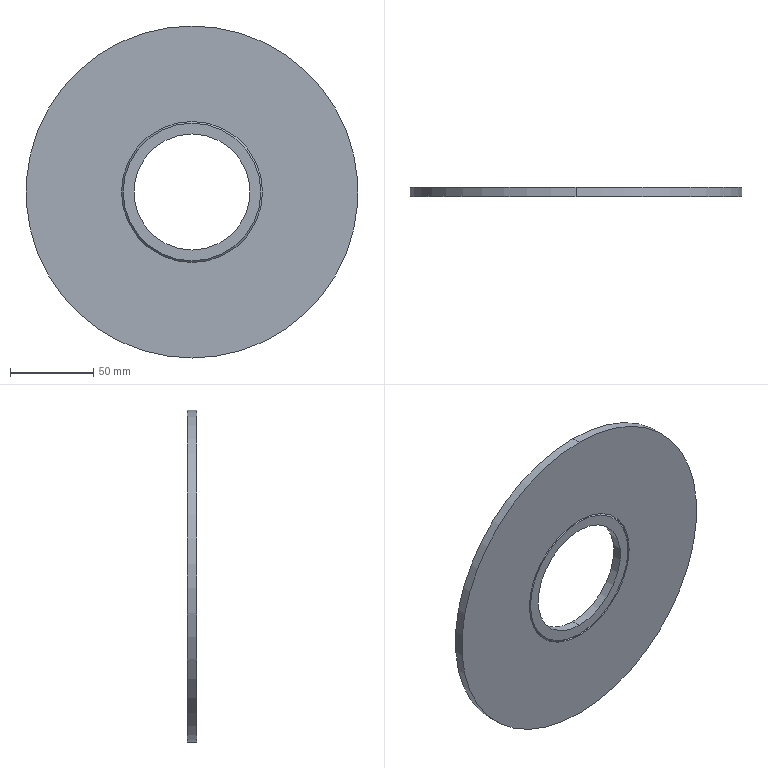Part | SolidWorks | features Chamfer 1, Extrusion 1, ICE 1 | 1 solid | 16 faces | box 200 x 5.5 x 200 mm | volume 151356 mm3 | cylinder 8 | cone 4 | plane 4 | commonest cylinder face diameters 85 x4 70 x2 200 x2
STEP:
#1=CARTESIAN_POINT('',(0.,4.5,42.5));
#2=VERTEX_POINT('',#1);
#3=CARTESIAN_POINT('',(0.,4.5,-42.5));
#4=VERTEX_POINT('',#3);
#5=CARTESIAN_POINT('',(0.,4.5,0.));
#6=DIRECTION('',(0.,-1.,0.));
#7=DIRECTION('',(0.,0.,1.));
#8=AXIS2_PLACEMENT_3D('',#5,#6,#7);
#9=CIRCLE('',#8,42.5);
#10=EDGE_CURVE('',#2,#4,#9,.T.);
#11=ORIENTED_EDGE('',*,*,#10,.T.);
#12=CARTESIAN_POINT('',(0.,5.5,-42.5));
#13=VERTEX_POINT('',#12);
#14=CARTESIAN_POINT('',(0.,0.,-42.5));
#15=DIRECTION('',(0.,1.,0.));
#16=VECTOR('',#15,1000.);
#17=LINE('',#14,#16);
#18=EDGE_CURVE('',#4,#13,#17,.T.);
#19=ORIENTED_EDGE('',*,*,#18,.T.);
#20=CARTESIAN_POINT('',(0.,5.5,42.5));
#21=VERTEX_POINT('',#20);
#22=CARTESIAN_POINT('',(0.,5.5,0.));
#23=DIRECTION('',(0.,1.,0.));
#24=DIRECTION('',(0.,0.,1.));
#25=AXIS2_PLACEMENT_3D('',#22,#23,#24);
#26=CIRCLE('',#25,42.5);
#27=EDGE_CURVE('',#13,#21,#26,.T.);
#28=ORIENTED_EDGE('',*,*,#27,.T.);
#29=CARTESIAN_POINT('',(0.,0.,42.5));
#30=DIRECTION('',(0.,1.,0.));
#31=VECTOR('',#30,1000.);
#32=LINE('',#29,#31);
#33=EDGE_CURVE('',#2,#21,#32,.T.);
#34=ORIENTED_EDGE('',*,*,#33,.F.);
#35=EDGE_LOOP('',(#11,#19,#28,#34));
#36=FACE_OUTER_BOUND('',#35,.T.);
#37=CARTESIAN_POINT('',(0.,0.,0.));
#38=DIRECTION('',(0.,1.,0.));
#39=DIRECTION('',(0.,0.,1.));
#40=AXIS2_PLACEMENT_3D('',#37,#38,#39);
#41=CYLINDRICAL_SURFACE('',#40,42.5);
#42=ADVANCED_FACE('',(#36),#41,.F.);
#43=CARTESIAN_POINT('',(0.,0.,100.));
#44=VERTEX_POINT('',#43);
#45=CARTESIAN_POINT('',(0.,0.,-100.));
#46=VERTEX_POINT('',#45);
#47=CARTESIAN_POINT('',(0.,0.,0.));
#48=DIRECTION('',(0.,1.,0.));
#49=DIRECTION('',(0.,0.,1.));
#50=AXIS2_PLACEMENT_3D('',#47,#48,#49);
#51=CIRCLE('',#50,100.);
#52=EDGE_CURVE('',#44,#46,#51,.T.);
#53=ORIENTED_EDGE('',*,*,#52,.T.);
#54=CARTESIAN_POINT('',(0.,5.5,-100.));
#55=VERTEX_POINT('',#54);
#56=CARTESIAN_POINT('',(0.,0.,-100.));
#57=DIRECTION('',(0.,1.,0.));
#58=VECTOR('',#57,1000.);
#59=LINE('',#56,#58);
#60=EDGE_CURVE('',#46,#55,#59,.T.);
#61=ORIENTED_EDGE('',*,*,#60,.T.);
#62=CARTESIAN_POINT('',(0.,5.5,100.));
#63=VERTEX_POINT('',#62);
#64=CARTESIAN_POINT('',(0.,5.5,0.));
#65=DIRECTION('',(0.,1.,0.));
#66=DIRECTION('',(0.,0.,1.));
#67=AXIS2_PLACEMENT_3D('',#64,#65,#66);
#68=CIRCLE('',#67,100.);
#69=EDGE_CURVE('',#63,#55,#68,.T.);
#70=ORIENTED_EDGE('',*,*,#69,.F.);
#71=CARTESIAN_POINT('',(0.,0.,100.));
#72=DIRECTION('',(0.,1.,0.));
#73=VECTOR('',#72,1000.);
#74=LINE('',#71,#73);
#75=EDGE_CURVE('',#44,#63,#74,.T.);
#76=ORIENTED_EDGE('',*,*,#75,.F.);
#77=EDGE_LOOP('',(#53,#61,#70,#76));
#78=FACE_OUTER_BOUND('',#77,.T.);
#79=CARTESIAN_POINT('',(0.,0.,0.));
#80=DIRECTION('',(0.,1.,0.));
#81=DIRECTION('',(0.,0.,1.));
#82=AXIS2_PLACEMENT_3D('',#79,#80,#81);
#83=CYLINDRICAL_SURFACE('',#82,100.);
#84=ADVANCED_FACE('',(#78),#83,.T.);
#85=CARTESIAN_POINT('',(0.,0.,-42.5));
#86=VERTEX_POINT('',#85);
#87=CARTESIAN_POINT('',(0.,0.,42.5));
#88=VERTEX_POINT('',#87);
#89=CARTESIAN_POINT('',(0.,0.,0.));
#90=DIRECTION('',(0.,1.,0.));
#91=DIRECTION('',(0.,0.,1.));
#92=AXIS2_PLACEMENT_3D('',#89,#90,#91);
#93=CIRCLE('',#92,42.5);
#94=EDGE_CURVE('',#86,#88,#93,.T.);
#95=ORIENTED_EDGE('',*,*,#94,.F.);
#96=CARTESIAN_POINT('',(0.,1.,-42.5));
#97=VERTEX_POINT('',#96);
#98=CARTESIAN_POINT('',(0.,0.,-42.5));
#99=DIRECTION('',(0.,1.,0.));
#100=VECTOR('',#99,1000.);
#101=LINE('',#98,#100);
#102=EDGE_CURVE('',#86,#97,#101,.T.);
#103=ORIENTED_EDGE('',*,*,#102,.T.);
#104=CARTESIAN_POINT('',(0.,1.,42.5));
#105=VERTEX_POINT('',#104);
#106=CARTESIAN_POINT('',(0.,1.,0.));
#107=DIRECTION('',(0.,1.,0.));
#108=DIRECTION('',(0.,0.,1.));
#109=AXIS2_PLACEMENT_3D('',#106,#107,#108);
#110=CIRCLE('',#109,42.5);
#111=EDGE_CURVE('',#97,#105,#110,.T.);
#112=ORIENTED_EDGE('',*,*,#111,.T.);
#113=CARTESIAN_POINT('',(0.,0.,42.5));
#114=DIRECTION('',(0.,1.,0.));
#115=VECTOR('',#114,1000.);
#116=LINE('',#113,#115);
#117=EDGE_CURVE('',#88,#105,#116,.T.);
#118=ORIENTED_EDGE('',*,*,#117,.F.);
#119=EDGE_LOOP('',(#95,#103,#112,#118));
#120=FACE_OUTER_BOUND('',#119,.T.);
#121=CARTESIAN_POINT('',(0.,0.,0.));
#122=DIRECTION('',(0.,1.,0.));
#123=DIRECTION('',(0.,0.,1.));
#124=AXIS2_PLACEMENT_3D('',#121,#122,#123);
#125=CYLINDRICAL_SURFACE('',#124,42.5);
#126=ADVANCED_FACE('',(#120),#125,.F.);
#127=CARTESIAN_POINT('',(0.,5.5,41.5));
#128=VERTEX_POINT('',#127);
#129=CARTESIAN_POINT('',(0.,5.5,-41.5));
#130=VERTEX_POINT('',#129);
#131=CARTESIAN_POINT('',(0.,5.5,0.));
#132=DIRECTION('',(0.,1.,0.));
#133=DIRECTION('',(0.,0.,1.));
#134=AXIS2_PLACEMENT_3D('',#131,#132,#133);
#135=CIRCLE('',#134,41.5);
#136=EDGE_CURVE('',#128,#130,#135,.T.);
#137=ORIENTED_EDGE('',*,*,#136,.F.);
#138=CARTESIAN_POINT('',(0.,5.5,41.5));
#139=DIRECTION('',(0.,-0.7071,0.7071));
#140=VECTOR('',#139,1000.);
#141=LINE('',#138,#140);
#142=EDGE_CURVE('',#128,#2,#141,.T.);
#143=ORIENTED_EDGE('',*,*,#142,.T.);
#144=CARTESIAN_POINT('',(0.,4.5,0.));
#145=DIRECTION('',(0.,-1.,0.));
#146=DIRECTION('',(0.,0.,1.));
#147=AXIS2_PLACEMENT_3D('',#144,#145,#146);
#148=CIRCLE('',#147,42.5);
#149=EDGE_CURVE('',#4,#2,#148,.T.);
#150=ORIENTED_EDGE('',*,*,#149,.F.);
#151=CARTESIAN_POINT('',(0.,5.5,-41.5));
#152=DIRECTION('',(0.,-0.7071,-0.7071));
#153=VECTOR('',#152,1000.);
#154=LINE('',#151,#153);
#155=EDGE_CURVE('',#130,#4,#154,.T.);
#156=ORIENTED_EDGE('',*,*,#155,.F.);
#157=EDGE_LOOP('',(#137,#143,#150,#156));
#158=FACE_OUTER_BOUND('',#157,.T.);
#159=CARTESIAN_POINT('',(0.,5.5,0.));
#160=DIRECTION('',(0.,-1.,0.));
#161=DIRECTION('',(0.,0.,-1.));
#162=AXIS2_PLACEMENT_3D('',#159,#160,#161);
#163=CONICAL_SURFACE('',#162,41.5,0.7854);
#164=ADVANCED_FACE('',(#158),#163,.T.);
#165=CARTESIAN_POINT('',(0.,0.,-41.5));
#166=VERTEX_POINT('',#165);
#167=CARTESIAN_POINT('',(0.,0.,41.5));
#168=VERTEX_POINT('',#167);
#169=CARTESIAN_POINT('',(0.,0.,0.));
#170=DIRECTION('',(0.,-1.,0.));
#171=DIRECTION('',(0.,0.,1.));
#172=AXIS2_PLACEMENT_3D('',#169,#170,#171);
#173=CIRCLE('',#172,41.5);
#174=EDGE_CURVE('',#166,#168,#173,.T.);
#175=ORIENTED_EDGE('',*,*,#174,.F.);
#176=CARTESIAN_POINT('',(0.,1.,-42.5));
#177=DIRECTION('',(0.,0.7071,-0.7071));
#178=VECTOR('',#177,1000.);
#179=LINE('',#176,#178);
#180=EDGE_CURVE('',#166,#97,#179,.T.);
#181=ORIENTED_EDGE('',*,*,#180,.T.);
#182=CARTESIAN_POINT('',(0.,1.,0.));
#183=DIRECTION('',(0.,1.,0.));
#184=DIRECTION('',(0.,0.,1.));
#185=AXIS2_PLACEMENT_3D('',#182,#183,#184);
#186=CIRCLE('',#185,42.5);
#187=EDGE_CURVE('',#105,#97,#186,.T.);
#188=ORIENTED_EDGE('',*,*,#187,.F.);
#189=CARTESIAN_POINT('',(0.,1.,42.5));
#190=DIRECTION('',(0.,0.7071,0.7071));
#191=VECTOR('',#190,1000.);
#192=LINE('',#189,#191);
#193=EDGE_CURVE('',#168,#105,#192,.T.);
#194=ORIENTED_EDGE('',*,*,#193,.F.);
#195=EDGE_LOOP('',(#175,#181,#188,#194));
#196=FACE_OUTER_BOUND('',#195,.T.);
#197=CARTESIAN_POINT('',(0.,1.,0.));
#198=DIRECTION('',(0.,1.,0.));
#199=DIRECTION('',(0.,0.,1.));
#200=AXIS2_PLACEMENT_3D('',#197,#198,#199);
#201=CONICAL_SURFACE('',#200,42.5,0.7854);
#202=ADVANCED_FACE('',(#196),#201,.T.);
#203=CARTESIAN_POINT('',(0.,5.5,-35.));
#204=VERTEX_POINT('',#203);
#205=CARTESIAN_POINT('',(0.,5.5,35.));
#206=VERTEX_POINT('',#205);
#207=CARTESIAN_POINT('',(0.,5.5,0.));
#208=DIRECTION('',(0.,1.,0.));
#209=DIRECTION('',(0.,0.,1.));
#210=AXIS2_PLACEMENT_3D('',#207,#208,#209);
#211=CIRCLE('',#210,35.);
#212=EDGE_CURVE('',#204,#206,#211,.T.);
#213=ORIENTED_EDGE('',*,*,#212,.T.);
#214=CARTESIAN_POINT('',(0.,0.,35.));
#215=VERTEX_POINT('',#214);
#216=CARTESIAN_POINT('',(0.,5.5,35.));
#217=DIRECTION('',(0.,-1.,0.));
#218=VECTOR('',#217,1000.);
#219=LINE('',#216,#218);
#220=EDGE_CURVE('',#206,#215,#219,.T.);
#221=ORIENTED_EDGE('',*,*,#220,.T.);
#222=CARTESIAN_POINT('',(0.,0.,-35.));
#223=VERTEX_POINT('',#222);
#224=CARTESIAN_POINT('',(0.,0.,0.));
#225=DIRECTION('',(0.,1.,0.));
#226=DIRECTION('',(0.,0.,1.));
#227=AXIS2_PLACEMENT_3D('',#224,#225,#226);
#228=CIRCLE('',#227,35.);
#229=EDGE_CURVE('',#223,#215,#228,.T.);
#230=ORIENTED_EDGE('',*,*,#229,.F.);
#231=CARTESIAN_POINT('',(0.,5.5,-35.));
#232=DIRECTION('',(0.,-1.,0.));
#233=VECTOR('',#232,1000.);
#234=LINE('',#231,#233);
#235=EDGE_CURVE('',#204,#223,#234,.T.);
#236=ORIENTED_EDGE('',*,*,#235,.F.);
#237=EDGE_LOOP('',(#213,#221,#230,#236));
#238=FACE_OUTER_BOUND('',#237,.T.);
#239=CARTESIAN_POINT('',(0.,5.5,0.));
#240=DIRECTION('',(0.,-1.,0.));
#241=DIRECTION('',(0.,0.,-1.));
#242=AXIS2_PLACEMENT_3D('',#239,#240,#241);
#243=CYLINDRICAL_SURFACE('',#242,35.);
#244=ADVANCED_FACE('',(#238),#243,.F.);
#245=CARTESIAN_POINT('',(0.,5.5,0.));
#246=DIRECTION('',(0.,1.,0.));
#247=DIRECTION('',(0.,0.,1.));
#248=AXIS2_PLACEMENT_3D('',#245,#246,#247);
#249=CIRCLE('',#248,41.5);
#250=EDGE_CURVE('',#130,#128,#249,.T.);
#251=ORIENTED_EDGE('',*,*,#250,.T.);
#252=ORIENTED_EDGE('',*,*,#136,.T.);
#253=EDGE_LOOP('',(#251,#252));
#254=FACE_OUTER_BOUND('',#253,.T.);
#255=ORIENTED_EDGE('',*,*,#212,.F.);
#256=CARTESIAN_POINT('',(0.,5.5,0.));
#257=DIRECTION('',(0.,1.,0.));
#258=DIRECTION('',(0.,0.,1.));
#259=AXIS2_PLACEMENT_3D('',#256,#257,#258);
#260=CIRCLE('',#259,35.);
#261=EDGE_CURVE('',#206,#204,#260,.T.);
#262=ORIENTED_EDGE('',*,*,#261,.F.);
#263=EDGE_LOOP('',(#255,#262));
#264=FACE_BOUND('',#263,.T.);
#265=CARTESIAN_POINT('',(0.,5.5,0.));
#266=DIRECTION('',(0.,1.,0.));
#267=DIRECTION('',(0.,0.,1.));
#268=AXIS2_PLACEMENT_3D('',#265,#266,#267);
#269=PLANE('',#268);
#270=ADVANCED_FACE('',(#254,#264),#269,.T.);
#271=CARTESIAN_POINT('',(0.,0.,0.));
#272=DIRECTION('',(0.,-1.,0.));
#273=DIRECTION('',(0.,0.,1.));
#274=AXIS2_PLACEMENT_3D('',#271,#272,#273);
#275=CIRCLE('',#274,41.5);
#276=EDGE_CURVE('',#168,#166,#275,.T.);
#277=ORIENTED_EDGE('',*,*,#276,.T.);
#278=ORIENTED_EDGE('',*,*,#174,.T.);
#279=EDGE_LOOP('',(#277,#278));
#280=FACE_OUTER_BOUND('',#279,.T.);
#281=ORIENTED_EDGE('',*,*,#229,.T.);
#282=CARTESIAN_POINT('',(0.,0.,0.));
#283=DIRECTION('',(0.,1.,0.));
#284=DIRECTION('',(0.,0.,1.));
#285=AXIS2_PLACEMENT_3D('',#282,#283,#284);
#286=CIRCLE('',#285,35.);
#287=EDGE_CURVE('',#215,#223,#286,.T.);
#288=ORIENTED_EDGE('',*,*,#287,.T.);
#289=EDGE_LOOP('',(#281,#288));
#290=FACE_BOUND('',#289,.T.);
#291=CARTESIAN_POINT('',(0.,0.,0.));
#292=DIRECTION('',(0.,1.,0.));
#293=DIRECTION('',(0.,0.,1.));
#294=AXIS2_PLACEMENT_3D('',#291,#292,#293);
#295=PLANE('',#294);
#296=ADVANCED_FACE('',(#280,#290),#295,.F.);
#297=ORIENTED_EDGE('',*,*,#220,.F.);
#298=ORIENTED_EDGE('',*,*,#261,.T.);
#299=ORIENTED_EDGE('',*,*,#235,.T.);
#300=ORIENTED_EDGE('',*,*,#287,.F.);
#301=EDGE_LOOP('',(#297,#298,#299,#300));
#302=FACE_OUTER_BOUND('',#301,.T.);
#303=CARTESIAN_POINT('',(0.,5.5,0.));
#304=DIRECTION('',(0.,-1.,0.));
#305=DIRECTION('',(0.,0.,-1.));
#306=AXIS2_PLACEMENT_3D('',#303,#304,#305);
#307=CYLINDRICAL_SURFACE('',#306,35.);
#308=ADVANCED_FACE('',(#302),#307,.F.);
#309=ORIENTED_EDGE('',*,*,#180,.F.);
#310=ORIENTED_EDGE('',*,*,#276,.F.);
#311=ORIENTED_EDGE('',*,*,#193,.T.);
#312=ORIENTED_EDGE('',*,*,#111,.F.);
#313=EDGE_LOOP('',(#309,#310,#311,#312));
#314=FACE_OUTER_BOUND('',#313,.T.);
#315=CARTESIAN_POINT('',(0.,1.,0.));
#316=DIRECTION('',(0.,1.,0.));
#317=DIRECTION('',(0.,0.,1.));
#318=AXIS2_PLACEMENT_3D('',#315,#316,#317);
#319=CONICAL_SURFACE('',#318,42.5,0.7854);
#320=ADVANCED_FACE('',(#314),#319,.T.);
#321=ORIENTED_EDGE('',*,*,#142,.F.);
#322=ORIENTED_EDGE('',*,*,#250,.F.);
#323=ORIENTED_EDGE('',*,*,#155,.T.);
#324=ORIENTED_EDGE('',*,*,#10,.F.);
#325=EDGE_LOOP('',(#321,#322,#323,#324));
#326=FACE_OUTER_BOUND('',#325,.T.);
#327=CARTESIAN_POINT('',(0.,5.5,0.));
#328=DIRECTION('',(0.,-1.,0.));
#329=DIRECTION('',(0.,0.,-1.));
#330=AXIS2_PLACEMENT_3D('',#327,#328,#329);
#331=CONICAL_SURFACE('',#330,41.5,0.7854);
#332=ADVANCED_FACE('',(#326),#331,.T.);
#333=ORIENTED_EDGE('',*,*,#102,.F.);
#334=CARTESIAN_POINT('',(0.,0.,0.));
#335=DIRECTION('',(0.,1.,0.));
#336=DIRECTION('',(0.,0.,1.));
#337=AXIS2_PLACEMENT_3D('',#334,#335,#336);
#338=CIRCLE('',#337,42.5);
#339=EDGE_CURVE('',#88,#86,#338,.T.);
#340=ORIENTED_EDGE('',*,*,#339,.F.);
#341=ORIENTED_EDGE('',*,*,#117,.T.);
#342=ORIENTED_EDGE('',*,*,#187,.T.);
#343=EDGE_LOOP('',(#333,#340,#341,#342));
#344=FACE_OUTER_BOUND('',#343,.T.);
#345=CARTESIAN_POINT('',(0.,0.,0.));
#346=DIRECTION('',(0.,1.,0.));
#347=DIRECTION('',(0.,0.,1.));
#348=AXIS2_PLACEMENT_3D('',#345,#346,#347);
#349=CYLINDRICAL_SURFACE('',#348,42.5);
#350=ADVANCED_FACE('',(#344),#349,.F.);
#351=ORIENTED_EDGE('',*,*,#60,.F.);
#352=CARTESIAN_POINT('',(0.,0.,0.));
#353=DIRECTION('',(0.,1.,0.));
#354=DIRECTION('',(0.,0.,1.));
#355=AXIS2_PLACEMENT_3D('',#352,#353,#354);
#356=CIRCLE('',#355,100.);
#357=EDGE_CURVE('',#46,#44,#356,.T.);
#358=ORIENTED_EDGE('',*,*,#357,.T.);
#359=ORIENTED_EDGE('',*,*,#75,.T.);
#360=CARTESIAN_POINT('',(0.,5.5,0.));
#361=DIRECTION('',(0.,1.,0.));
#362=DIRECTION('',(0.,0.,1.));
#363=AXIS2_PLACEMENT_3D('',#360,#361,#362);
#364=CIRCLE('',#363,100.);
#365=EDGE_CURVE('',#55,#63,#364,.T.);
#366=ORIENTED_EDGE('',*,*,#365,.F.);
#367=EDGE_LOOP('',(#351,#358,#359,#366));
#368=FACE_OUTER_BOUND('',#367,.T.);
#369=CARTESIAN_POINT('',(0.,0.,0.));
#370=DIRECTION('',(0.,1.,0.));
#371=DIRECTION('',(0.,0.,1.));
#372=AXIS2_PLACEMENT_3D('',#369,#370,#371);
#373=CYLINDRICAL_SURFACE('',#372,100.);
#374=ADVANCED_FACE('',(#368),#373,.T.);
#375=ORIENTED_EDGE('',*,*,#339,.T.);
#376=ORIENTED_EDGE('',*,*,#94,.T.);
#377=EDGE_LOOP('',(#375,#376));
#378=FACE_BOUND('',#377,.T.);
#379=ORIENTED_EDGE('',*,*,#52,.F.);
#380=ORIENTED_EDGE('',*,*,#357,.F.);
#381=EDGE_LOOP('',(#379,#380));
#382=FACE_OUTER_BOUND('',#381,.T.);
#383=CARTESIAN_POINT('',(0.,0.,0.));
#384=DIRECTION('',(0.,1.,0.));
#385=DIRECTION('',(0.,0.,1.));
#386=AXIS2_PLACEMENT_3D('',#383,#384,#385);
#387=PLANE('',#386);
#388=ADVANCED_FACE('',(#378,#382),#387,.F.);
#389=CARTESIAN_POINT('',(0.,5.5,0.));
#390=DIRECTION('',(0.,1.,0.));
#391=DIRECTION('',(0.,0.,1.));
#392=AXIS2_PLACEMENT_3D('',#389,#390,#391);
#393=CIRCLE('',#392,42.5);
#394=EDGE_CURVE('',#21,#13,#393,.T.);
#395=ORIENTED_EDGE('',*,*,#394,.F.);
#396=ORIENTED_EDGE('',*,*,#27,.F.);
#397=EDGE_LOOP('',(#395,#396));
#398=FACE_BOUND('',#397,.T.);
#399=ORIENTED_EDGE('',*,*,#69,.T.);
#400=ORIENTED_EDGE('',*,*,#365,.T.);
#401=EDGE_LOOP('',(#399,#400));
#402=FACE_OUTER_BOUND('',#401,.T.);
#403=CARTESIAN_POINT('',(0.,5.5,0.));
#404=DIRECTION('',(0.,1.,0.));
#405=DIRECTION('',(0.,0.,1.));
#406=AXIS2_PLACEMENT_3D('',#403,#404,#405);
#407=PLANE('',#406);
#408=ADVANCED_FACE('',(#398,#402),#407,.T.);
#409=ORIENTED_EDGE('',*,*,#18,.F.);
#410=ORIENTED_EDGE('',*,*,#149,.T.);
#411=ORIENTED_EDGE('',*,*,#33,.T.);
#412=ORIENTED_EDGE('',*,*,#394,.T.);
#413=EDGE_LOOP('',(#409,#410,#411,#412));
#414=FACE_OUTER_BOUND('',#413,.T.);
#415=CARTESIAN_POINT('',(0.,0.,0.));
#416=DIRECTION('',(0.,1.,0.));
#417=DIRECTION('',(0.,0.,1.));
#418=AXIS2_PLACEMENT_3D('',#415,#416,#417);
#419=CYLINDRICAL_SURFACE('',#418,42.5);
#420=ADVANCED_FACE('',(#414),#419,.F.);
#421=CLOSED_SHELL('',(#42,#84,#126,#164,#202,#244,#270,#296,#308,#320,#332,#350,#374,#388,#408,#420));
#422=MANIFOLD_SOLID_BREP('',#421);
#423=CARTESIAN_POINT('',(0.,0.,0.));
#424=DIRECTION('',(0.,0.,1.));
#425=DIRECTION('',(1.,0.,0.));
#426=AXIS2_PLACEMENT_3D('',#423,#424,#425);
#427=(LENGTH_UNIT()NAMED_UNIT(*)SI_UNIT(.MILLI.,.METRE.));
#428=UNCERTAINTY_MEASURE_WITH_UNIT(LENGTH_MEASURE(0.00001),#427,'','');
#429=(NAMED_UNIT(*)PLANE_ANGLE_UNIT()SI_UNIT($,.RADIAN.));
#430=(NAMED_UNIT(*)SI_UNIT($,.STERADIAN.)SOLID_ANGLE_UNIT());
#431=(GEOMETRIC_REPRESENTATION_CONTEXT(3)GLOBAL_UNCERTAINTY_ASSIGNED_CONTEXT((#428))GLOBAL_UNIT_ASSIGNED_CONTEXT((#427,#429,#430))REPRESENTATION_CONTEXT('',''));
#432=ADVANCED_BREP_SHAPE_REPRESENTATION('',(#422,#426),#431);